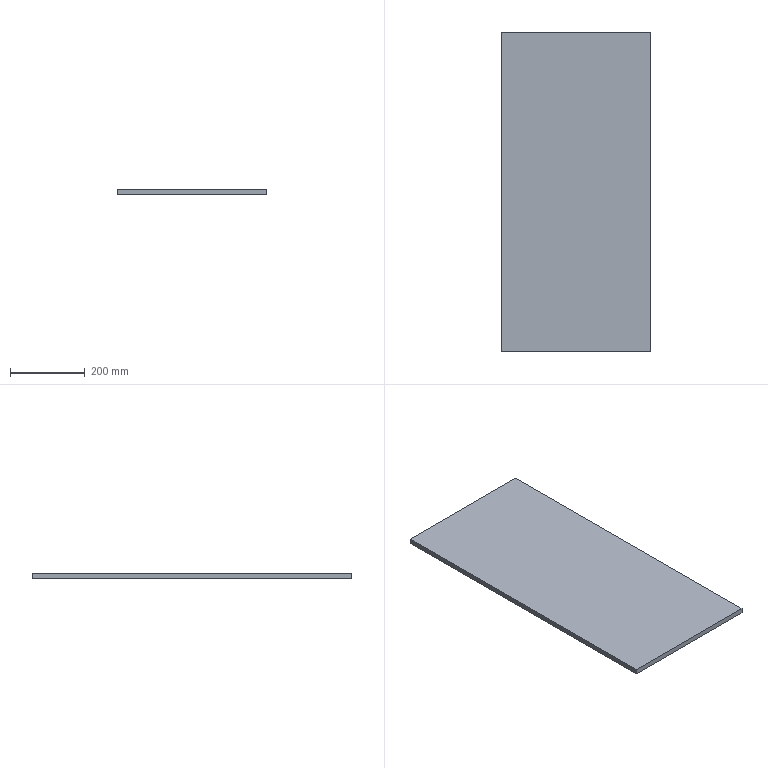Part | SolidWorks | features Extrusion 1 | 1 solid | 6 faces | box 400 x 855 x 14 mm | volume 4788000 mm3 | plane 6
STEP:
#1=CARTESIAN_POINT('',(-200.,427.5,-7.));
#2=VERTEX_POINT('',#1);
#3=CARTESIAN_POINT('',(-200.,-427.5,-7.));
#4=VERTEX_POINT('',#3);
#5=CARTESIAN_POINT('',(-200.,427.5,-7.));
#6=DIRECTION('',(0.,-1.,0.));
#7=VECTOR('',#6,1000.);
#8=LINE('',#5,#7);
#9=EDGE_CURVE('',#2,#4,#8,.T.);
#10=ORIENTED_EDGE('',*,*,#9,.T.);
#11=CARTESIAN_POINT('',(-200.,-427.5,7.));
#12=VERTEX_POINT('',#11);
#13=CARTESIAN_POINT('',(-200.,-427.5,7.));
#14=DIRECTION('',(0.,0.,-1.));
#15=VECTOR('',#14,1000.);
#16=LINE('',#13,#15);
#17=EDGE_CURVE('',#12,#4,#16,.T.);
#18=ORIENTED_EDGE('',*,*,#17,.F.);
#19=CARTESIAN_POINT('',(-200.,427.5,7.));
#20=VERTEX_POINT('',#19);
#21=CARTESIAN_POINT('',(-200.,427.5,7.));
#22=DIRECTION('',(0.,-1.,0.));
#23=VECTOR('',#22,1000.);
#24=LINE('',#21,#23);
#25=EDGE_CURVE('',#20,#12,#24,.T.);
#26=ORIENTED_EDGE('',*,*,#25,.F.);
#27=CARTESIAN_POINT('',(-200.,427.5,7.));
#28=DIRECTION('',(0.,0.,-1.));
#29=VECTOR('',#28,1000.);
#30=LINE('',#27,#29);
#31=EDGE_CURVE('',#20,#2,#30,.T.);
#32=ORIENTED_EDGE('',*,*,#31,.T.);
#33=EDGE_LOOP('',(#10,#18,#26,#32));
#34=FACE_OUTER_BOUND('',#33,.T.);
#35=CARTESIAN_POINT('',(-200.,427.5,7.));
#36=DIRECTION('',(1.,0.,0.));
#37=DIRECTION('',(0.,1.,0.));
#38=AXIS2_PLACEMENT_3D('',#35,#36,#37);
#39=PLANE('',#38);
#40=ADVANCED_FACE('',(#34),#39,.F.);
#41=CARTESIAN_POINT('',(200.,-427.5,-7.));
#42=VERTEX_POINT('',#41);
#43=CARTESIAN_POINT('',(-200.,-427.5,-7.));
#44=DIRECTION('',(1.,0.,0.));
#45=VECTOR('',#44,1000.);
#46=LINE('',#43,#45);
#47=EDGE_CURVE('',#4,#42,#46,.T.);
#48=ORIENTED_EDGE('',*,*,#47,.T.);
#49=CARTESIAN_POINT('',(200.,-427.5,7.));
#50=VERTEX_POINT('',#49);
#51=CARTESIAN_POINT('',(200.,-427.5,7.));
#52=DIRECTION('',(0.,0.,-1.));
#53=VECTOR('',#52,1000.);
#54=LINE('',#51,#53);
#55=EDGE_CURVE('',#50,#42,#54,.T.);
#56=ORIENTED_EDGE('',*,*,#55,.F.);
#57=CARTESIAN_POINT('',(-200.,-427.5,7.));
#58=DIRECTION('',(1.,0.,0.));
#59=VECTOR('',#58,1000.);
#60=LINE('',#57,#59);
#61=EDGE_CURVE('',#12,#50,#60,.T.);
#62=ORIENTED_EDGE('',*,*,#61,.F.);
#63=ORIENTED_EDGE('',*,*,#17,.T.);
#64=EDGE_LOOP('',(#48,#56,#62,#63));
#65=FACE_OUTER_BOUND('',#64,.T.);
#66=CARTESIAN_POINT('',(-200.,-427.5,7.));
#67=DIRECTION('',(0.,1.,0.));
#68=DIRECTION('',(0.,0.,1.));
#69=AXIS2_PLACEMENT_3D('',#66,#67,#68);
#70=PLANE('',#69);
#71=ADVANCED_FACE('',(#65),#70,.F.);
#72=CARTESIAN_POINT('',(200.,427.5,-7.));
#73=VERTEX_POINT('',#72);
#74=CARTESIAN_POINT('',(200.,427.5,-7.));
#75=DIRECTION('',(0.,1.,0.));
#76=VECTOR('',#75,1000.);
#77=LINE('',#74,#76);
#78=EDGE_CURVE('',#42,#73,#77,.T.);
#79=ORIENTED_EDGE('',*,*,#78,.T.);
#80=CARTESIAN_POINT('',(200.,427.5,7.));
#81=VERTEX_POINT('',#80);
#82=CARTESIAN_POINT('',(200.,427.5,7.));
#83=DIRECTION('',(0.,0.,-1.));
#84=VECTOR('',#83,1000.);
#85=LINE('',#82,#84);
#86=EDGE_CURVE('',#81,#73,#85,.T.);
#87=ORIENTED_EDGE('',*,*,#86,.F.);
#88=CARTESIAN_POINT('',(200.,427.5,7.));
#89=DIRECTION('',(0.,1.,0.));
#90=VECTOR('',#89,1000.);
#91=LINE('',#88,#90);
#92=EDGE_CURVE('',#50,#81,#91,.T.);
#93=ORIENTED_EDGE('',*,*,#92,.F.);
#94=ORIENTED_EDGE('',*,*,#55,.T.);
#95=EDGE_LOOP('',(#79,#87,#93,#94));
#96=FACE_OUTER_BOUND('',#95,.T.);
#97=CARTESIAN_POINT('',(200.,427.5,7.));
#98=DIRECTION('',(-1.,0.,0.));
#99=DIRECTION('',(0.,-1.,0.));
#100=AXIS2_PLACEMENT_3D('',#97,#98,#99);
#101=PLANE('',#100);
#102=ADVANCED_FACE('',(#96),#101,.F.);
#103=CARTESIAN_POINT('',(-200.,427.5,-7.));
#104=DIRECTION('',(-1.,0.,0.));
#105=VECTOR('',#104,1000.);
#106=LINE('',#103,#105);
#107=EDGE_CURVE('',#73,#2,#106,.T.);
#108=ORIENTED_EDGE('',*,*,#107,.T.);
#109=ORIENTED_EDGE('',*,*,#31,.F.);
#110=CARTESIAN_POINT('',(-200.,427.5,7.));
#111=DIRECTION('',(-1.,0.,0.));
#112=VECTOR('',#111,1000.);
#113=LINE('',#110,#112);
#114=EDGE_CURVE('',#81,#20,#113,.T.);
#115=ORIENTED_EDGE('',*,*,#114,.F.);
#116=ORIENTED_EDGE('',*,*,#86,.T.);
#117=EDGE_LOOP('',(#108,#109,#115,#116));
#118=FACE_OUTER_BOUND('',#117,.T.);
#119=CARTESIAN_POINT('',(-200.,427.5,7.));
#120=DIRECTION('',(0.,-1.,0.));
#121=DIRECTION('',(0.,0.,-1.));
#122=AXIS2_PLACEMENT_3D('',#119,#120,#121);
#123=PLANE('',#122);
#124=ADVANCED_FACE('',(#118),#123,.F.);
#125=ORIENTED_EDGE('',*,*,#25,.T.);
#126=ORIENTED_EDGE('',*,*,#61,.T.);
#127=ORIENTED_EDGE('',*,*,#92,.T.);
#128=ORIENTED_EDGE('',*,*,#114,.T.);
#129=EDGE_LOOP('',(#125,#126,#127,#128));
#130=FACE_OUTER_BOUND('',#129,.T.);
#131=CARTESIAN_POINT('',(-200.,-427.5,7.));
#132=DIRECTION('',(0.,0.,1.));
#133=DIRECTION('',(1.,0.,0.));
#134=AXIS2_PLACEMENT_3D('',#131,#132,#133);
#135=PLANE('',#134);
#136=ADVANCED_FACE('',(#130),#135,.T.);
#137=ORIENTED_EDGE('',*,*,#9,.F.);
#138=ORIENTED_EDGE('',*,*,#107,.F.);
#139=ORIENTED_EDGE('',*,*,#78,.F.);
#140=ORIENTED_EDGE('',*,*,#47,.F.);
#141=EDGE_LOOP('',(#137,#138,#139,#140));
#142=FACE_OUTER_BOUND('',#141,.T.);
#143=CARTESIAN_POINT('',(-200.,-427.5,-7.));
#144=DIRECTION('',(0.,0.,1.));
#145=DIRECTION('',(1.,0.,0.));
#146=AXIS2_PLACEMENT_3D('',#143,#144,#145);
#147=PLANE('',#146);
#148=ADVANCED_FACE('',(#142),#147,.F.);
#149=CLOSED_SHELL('',(#40,#71,#102,#124,#136,#148));
#150=MANIFOLD_SOLID_BREP('',#149);
#151=CARTESIAN_POINT('',(0.,0.,0.));
#152=DIRECTION('',(0.,0.,1.));
#153=DIRECTION('',(1.,0.,0.));
#154=AXIS2_PLACEMENT_3D('',#151,#152,#153);
#155=(LENGTH_UNIT()NAMED_UNIT(*)SI_UNIT(.MILLI.,.METRE.));
#156=UNCERTAINTY_MEASURE_WITH_UNIT(LENGTH_MEASURE(0.00001),#155,'','');
#157=(NAMED_UNIT(*)PLANE_ANGLE_UNIT()SI_UNIT($,.RADIAN.));
#158=(NAMED_UNIT(*)SI_UNIT($,.STERADIAN.)SOLID_ANGLE_UNIT());
#159=(GEOMETRIC_REPRESENTATION_CONTEXT(3)GLOBAL_UNCERTAINTY_ASSIGNED_CONTEXT((#156))GLOBAL_UNIT_ASSIGNED_CONTEXT((#155,#157,#158))REPRESENTATION_CONTEXT('',''));
#160=ADVANCED_BREP_SHAPE_REPRESENTATION('',(#150,#154),#159);